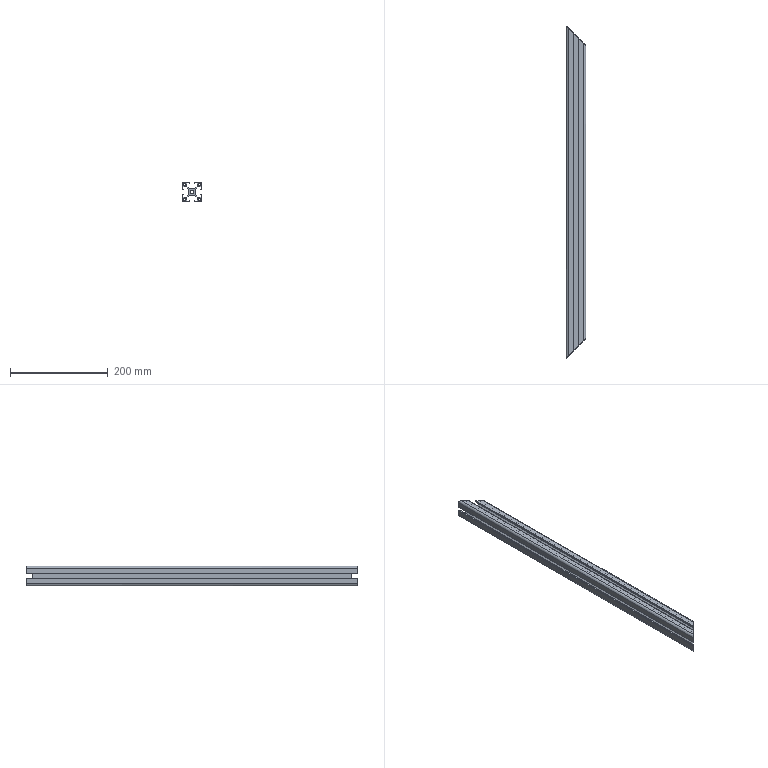Part | 1 solid | 104 faces | box 40 x 680 x 40 mm | volume 368990 mm3 | plane 94 | cylinder 10 | commonest cylinder face diameters 5 x4 9 x4 6.8 x2